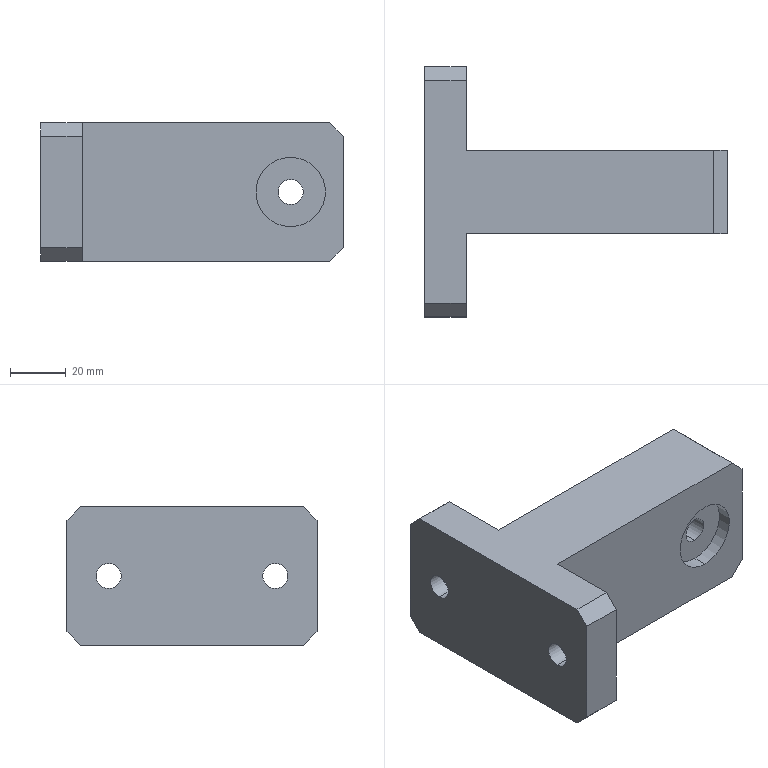Part | SolidWorks | features ICE 5, HoleWzd 3, Chamfer 1, Extrusion 1 | 1 solid | 31 faces | box 109 x 90 x 50 mm | volume 199011 mm3 | plane 19 | cylinder 12 | commonest cylinder face diameters 9 x6 15 x4 25 x2
STEP:
#1=CARTESIAN_POINT('',(6.,30.,7.5));
#2=VERTEX_POINT('',#1);
#3=CARTESIAN_POINT('',(6.,30.,-7.5));
#4=VERTEX_POINT('',#3);
#5=CARTESIAN_POINT('',(6.,30.,0.));
#6=DIRECTION('',(1.,0.,0.));
#7=DIRECTION('',(0.,0.,-1.));
#8=AXIS2_PLACEMENT_3D('',#5,#6,#7);
#9=CIRCLE('',#8,7.5);
#10=EDGE_CURVE('',#2,#4,#9,.T.);
#11=ORIENTED_EDGE('',*,*,#10,.F.);
#12=CARTESIAN_POINT('',(15.,30.,7.5));
#13=VERTEX_POINT('',#12);
#14=CARTESIAN_POINT('',(15.,30.,7.5));
#15=DIRECTION('',(1.,0.,0.));
#16=VECTOR('',#15,1000.);
#17=LINE('',#14,#16);
#18=EDGE_CURVE('',#2,#13,#17,.T.);
#19=ORIENTED_EDGE('',*,*,#18,.T.);
#20=CARTESIAN_POINT('',(15.,30.,-7.5));
#21=VERTEX_POINT('',#20);
#22=CARTESIAN_POINT('',(15.,30.,0.));
#23=DIRECTION('',(1.,0.,0.));
#24=DIRECTION('',(0.,0.,-1.));
#25=AXIS2_PLACEMENT_3D('',#22,#23,#24);
#26=CIRCLE('',#25,7.5);
#27=EDGE_CURVE('',#13,#21,#26,.T.);
#28=ORIENTED_EDGE('',*,*,#27,.T.);
#29=CARTESIAN_POINT('',(15.,30.,-7.5));
#30=DIRECTION('',(1.,0.,0.));
#31=VECTOR('',#30,1000.);
#32=LINE('',#29,#31);
#33=EDGE_CURVE('',#4,#21,#32,.T.);
#34=ORIENTED_EDGE('',*,*,#33,.F.);
#35=EDGE_LOOP('',(#11,#19,#28,#34));
#36=FACE_OUTER_BOUND('',#35,.T.);
#37=CARTESIAN_POINT('',(15.,30.,0.));
#38=DIRECTION('',(1.,0.,0.));
#39=DIRECTION('',(0.,0.,-1.));
#40=AXIS2_PLACEMENT_3D('',#37,#38,#39);
#41=CYLINDRICAL_SURFACE('',#40,7.5);
#42=ADVANCED_FACE('',(#36),#41,.F.);
#43=CARTESIAN_POINT('',(0.,30.,4.5));
#44=VERTEX_POINT('',#43);
#45=CARTESIAN_POINT('',(0.,30.,-4.5));
#46=VERTEX_POINT('',#45);
#47=CARTESIAN_POINT('',(0.,30.,0.));
#48=DIRECTION('',(1.,0.,0.));
#49=DIRECTION('',(0.,0.,-1.));
#50=AXIS2_PLACEMENT_3D('',#47,#48,#49);
#51=CIRCLE('',#50,4.5);
#52=EDGE_CURVE('',#44,#46,#51,.T.);
#53=ORIENTED_EDGE('',*,*,#52,.F.);
#54=CARTESIAN_POINT('',(6.,30.,4.5));
#55=VERTEX_POINT('',#54);
#56=CARTESIAN_POINT('',(15.,30.,4.5));
#57=DIRECTION('',(1.,0.,0.));
#58=VECTOR('',#57,1000.);
#59=LINE('',#56,#58);
#60=EDGE_CURVE('',#44,#55,#59,.T.);
#61=ORIENTED_EDGE('',*,*,#60,.T.);
#62=CARTESIAN_POINT('',(6.,30.,-4.5));
#63=VERTEX_POINT('',#62);
#64=CARTESIAN_POINT('',(6.,30.,0.));
#65=DIRECTION('',(1.,0.,0.));
#66=DIRECTION('',(0.,0.,-1.));
#67=AXIS2_PLACEMENT_3D('',#64,#65,#66);
#68=CIRCLE('',#67,4.5);
#69=EDGE_CURVE('',#55,#63,#68,.T.);
#70=ORIENTED_EDGE('',*,*,#69,.T.);
#71=CARTESIAN_POINT('',(15.,30.,-4.5));
#72=DIRECTION('',(1.,0.,0.));
#73=VECTOR('',#72,1000.);
#74=LINE('',#71,#73);
#75=EDGE_CURVE('',#46,#63,#74,.T.);
#76=ORIENTED_EDGE('',*,*,#75,.F.);
#77=EDGE_LOOP('',(#53,#61,#70,#76));
#78=FACE_OUTER_BOUND('',#77,.T.);
#79=CARTESIAN_POINT('',(15.,30.,0.));
#80=DIRECTION('',(1.,0.,0.));
#81=DIRECTION('',(0.,0.,-1.));
#82=AXIS2_PLACEMENT_3D('',#79,#80,#81);
#83=CYLINDRICAL_SURFACE('',#82,4.5);
#84=ADVANCED_FACE('',(#78),#83,.F.);
#85=CARTESIAN_POINT('',(6.,-30.,7.5));
#86=VERTEX_POINT('',#85);
#87=CARTESIAN_POINT('',(6.,-30.,-7.5));
#88=VERTEX_POINT('',#87);
#89=CARTESIAN_POINT('',(6.,-30.,0.));
#90=DIRECTION('',(1.,0.,0.));
#91=DIRECTION('',(0.,0.,-1.));
#92=AXIS2_PLACEMENT_3D('',#89,#90,#91);
#93=CIRCLE('',#92,7.5);
#94=EDGE_CURVE('',#86,#88,#93,.T.);
#95=ORIENTED_EDGE('',*,*,#94,.F.);
#96=CARTESIAN_POINT('',(15.,-30.,7.5));
#97=VERTEX_POINT('',#96);
#98=CARTESIAN_POINT('',(15.,-30.,7.5));
#99=DIRECTION('',(1.,0.,0.));
#100=VECTOR('',#99,1000.);
#101=LINE('',#98,#100);
#102=EDGE_CURVE('',#86,#97,#101,.T.);
#103=ORIENTED_EDGE('',*,*,#102,.T.);
#104=CARTESIAN_POINT('',(15.,-30.,-7.5));
#105=VERTEX_POINT('',#104);
#106=CARTESIAN_POINT('',(15.,-30.,0.));
#107=DIRECTION('',(1.,0.,0.));
#108=DIRECTION('',(0.,0.,-1.));
#109=AXIS2_PLACEMENT_3D('',#106,#107,#108);
#110=CIRCLE('',#109,7.5);
#111=EDGE_CURVE('',#97,#105,#110,.T.);
#112=ORIENTED_EDGE('',*,*,#111,.T.);
#113=CARTESIAN_POINT('',(15.,-30.,-7.5));
#114=DIRECTION('',(1.,0.,0.));
#115=VECTOR('',#114,1000.);
#116=LINE('',#113,#115);
#117=EDGE_CURVE('',#88,#105,#116,.T.);
#118=ORIENTED_EDGE('',*,*,#117,.F.);
#119=EDGE_LOOP('',(#95,#103,#112,#118));
#120=FACE_OUTER_BOUND('',#119,.T.);
#121=CARTESIAN_POINT('',(15.,-30.,0.));
#122=DIRECTION('',(1.,0.,0.));
#123=DIRECTION('',(0.,0.,-1.));
#124=AXIS2_PLACEMENT_3D('',#121,#122,#123);
#125=CYLINDRICAL_SURFACE('',#124,7.5);
#126=ADVANCED_FACE('',(#120),#125,.F.);
#127=CARTESIAN_POINT('',(0.,-30.,4.5));
#128=VERTEX_POINT('',#127);
#129=CARTESIAN_POINT('',(0.,-30.,-4.5));
#130=VERTEX_POINT('',#129);
#131=CARTESIAN_POINT('',(0.,-30.,0.));
#132=DIRECTION('',(1.,0.,0.));
#133=DIRECTION('',(0.,0.,-1.));
#134=AXIS2_PLACEMENT_3D('',#131,#132,#133);
#135=CIRCLE('',#134,4.5);
#136=EDGE_CURVE('',#128,#130,#135,.T.);
#137=ORIENTED_EDGE('',*,*,#136,.F.);
#138=CARTESIAN_POINT('',(6.,-30.,4.5));
#139=VERTEX_POINT('',#138);
#140=CARTESIAN_POINT('',(15.,-30.,4.5));
#141=DIRECTION('',(1.,0.,0.));
#142=VECTOR('',#141,1000.);
#143=LINE('',#140,#142);
#144=EDGE_CURVE('',#128,#139,#143,.T.);
#145=ORIENTED_EDGE('',*,*,#144,.T.);
#146=CARTESIAN_POINT('',(6.,-30.,-4.5));
#147=VERTEX_POINT('',#146);
#148=CARTESIAN_POINT('',(6.,-30.,0.));
#149=DIRECTION('',(1.,0.,0.));
#150=DIRECTION('',(0.,0.,-1.));
#151=AXIS2_PLACEMENT_3D('',#148,#149,#150);
#152=CIRCLE('',#151,4.5);
#153=EDGE_CURVE('',#139,#147,#152,.T.);
#154=ORIENTED_EDGE('',*,*,#153,.T.);
#155=CARTESIAN_POINT('',(15.,-30.,-4.5));
#156=DIRECTION('',(1.,0.,0.));
#157=VECTOR('',#156,1000.);
#158=LINE('',#155,#157);
#159=EDGE_CURVE('',#130,#147,#158,.T.);
#160=ORIENTED_EDGE('',*,*,#159,.F.);
#161=EDGE_LOOP('',(#137,#145,#154,#160));
#162=FACE_OUTER_BOUND('',#161,.T.);
#163=CARTESIAN_POINT('',(15.,-30.,0.));
#164=DIRECTION('',(1.,0.,0.));
#165=DIRECTION('',(0.,0.,-1.));
#166=AXIS2_PLACEMENT_3D('',#163,#164,#165);
#167=CYLINDRICAL_SURFACE('',#166,4.5);
#168=ADVANCED_FACE('',(#162),#167,.F.);
#169=CARTESIAN_POINT('',(90.,15.,4.5));
#170=VERTEX_POINT('',#169);
#171=CARTESIAN_POINT('',(90.,15.,-4.5));
#172=VERTEX_POINT('',#171);
#173=CARTESIAN_POINT('',(90.,15.,0.));
#174=DIRECTION('',(0.,-1.,0.));
#175=DIRECTION('',(0.,0.,-1.));
#176=AXIS2_PLACEMENT_3D('',#173,#174,#175);
#177=CIRCLE('',#176,4.5);
#178=EDGE_CURVE('',#170,#172,#177,.T.);
#179=ORIENTED_EDGE('',*,*,#178,.F.);
#180=CARTESIAN_POINT('',(90.,-10.,4.5));
#181=VERTEX_POINT('',#180);
#182=CARTESIAN_POINT('',(90.,-15.,4.5));
#183=DIRECTION('',(0.,-1.,0.));
#184=VECTOR('',#183,1000.);
#185=LINE('',#182,#184);
#186=EDGE_CURVE('',#170,#181,#185,.T.);
#187=ORIENTED_EDGE('',*,*,#186,.T.);
#188=CARTESIAN_POINT('',(90.,-10.,-4.5));
#189=VERTEX_POINT('',#188);
#190=CARTESIAN_POINT('',(90.,-10.,0.));
#191=DIRECTION('',(0.,-1.,0.));
#192=DIRECTION('',(0.,0.,-1.));
#193=AXIS2_PLACEMENT_3D('',#190,#191,#192);
#194=CIRCLE('',#193,4.5);
#195=EDGE_CURVE('',#181,#189,#194,.T.);
#196=ORIENTED_EDGE('',*,*,#195,.T.);
#197=CARTESIAN_POINT('',(90.,-15.,-4.5));
#198=DIRECTION('',(0.,-1.,0.));
#199=VECTOR('',#198,1000.);
#200=LINE('',#197,#199);
#201=EDGE_CURVE('',#172,#189,#200,.T.);
#202=ORIENTED_EDGE('',*,*,#201,.F.);
#203=EDGE_LOOP('',(#179,#187,#196,#202));
#204=FACE_OUTER_BOUND('',#203,.T.);
#205=CARTESIAN_POINT('',(90.,-15.,0.));
#206=DIRECTION('',(0.,-1.,0.));
#207=DIRECTION('',(0.,0.,-1.));
#208=AXIS2_PLACEMENT_3D('',#205,#206,#207);
#209=CYLINDRICAL_SURFACE('',#208,4.5);
#210=ADVANCED_FACE('',(#204),#209,.F.);
#211=CARTESIAN_POINT('',(90.,-10.,12.5));
#212=VERTEX_POINT('',#211);
#213=CARTESIAN_POINT('',(90.,-10.,-12.5));
#214=VERTEX_POINT('',#213);
#215=CARTESIAN_POINT('',(90.,-10.,0.));
#216=DIRECTION('',(0.,-1.,0.));
#217=DIRECTION('',(0.,0.,-1.));
#218=AXIS2_PLACEMENT_3D('',#215,#216,#217);
#219=CIRCLE('',#218,12.5);
#220=EDGE_CURVE('',#212,#214,#219,.T.);
#221=ORIENTED_EDGE('',*,*,#220,.F.);
#222=CARTESIAN_POINT('',(90.,-15.,12.5));
#223=VERTEX_POINT('',#222);
#224=CARTESIAN_POINT('',(90.,-10.,12.5));
#225=DIRECTION('',(0.,-1.,0.));
#226=VECTOR('',#225,1000.);
#227=LINE('',#224,#226);
#228=EDGE_CURVE('',#212,#223,#227,.T.);
#229=ORIENTED_EDGE('',*,*,#228,.T.);
#230=CARTESIAN_POINT('',(90.,-15.,-12.5));
#231=VERTEX_POINT('',#230);
#232=CARTESIAN_POINT('',(90.,-15.,0.));
#233=DIRECTION('',(0.,-1.,0.));
#234=DIRECTION('',(0.,0.,-1.));
#235=AXIS2_PLACEMENT_3D('',#232,#233,#234);
#236=CIRCLE('',#235,12.5);
#237=EDGE_CURVE('',#223,#231,#236,.T.);
#238=ORIENTED_EDGE('',*,*,#237,.T.);
#239=CARTESIAN_POINT('',(90.,-10.,-12.5));
#240=DIRECTION('',(0.,-1.,0.));
#241=VECTOR('',#240,1000.);
#242=LINE('',#239,#241);
#243=EDGE_CURVE('',#214,#231,#242,.T.);
#244=ORIENTED_EDGE('',*,*,#243,.F.);
#245=EDGE_LOOP('',(#221,#229,#238,#244));
#246=FACE_OUTER_BOUND('',#245,.T.);
#247=CARTESIAN_POINT('',(90.,-10.,0.));
#248=DIRECTION('',(0.,-1.,0.));
#249=DIRECTION('',(0.,0.,-1.));
#250=AXIS2_PLACEMENT_3D('',#247,#248,#249);
#251=CYLINDRICAL_SURFACE('',#250,12.5);
#252=ADVANCED_FACE('',(#246),#251,.F.);
#253=CARTESIAN_POINT('',(90.,15.,0.));
#254=DIRECTION('',(0.,-1.,0.));
#255=DIRECTION('',(0.,0.,-1.));
#256=AXIS2_PLACEMENT_3D('',#253,#254,#255);
#257=CIRCLE('',#256,4.5);
#258=EDGE_CURVE('',#172,#170,#257,.T.);
#259=ORIENTED_EDGE('',*,*,#258,.T.);
#260=ORIENTED_EDGE('',*,*,#178,.T.);
#261=EDGE_LOOP('',(#259,#260));
#262=FACE_BOUND('',#261,.T.);
#263=CARTESIAN_POINT('',(109.,15.,-20.));
#264=VERTEX_POINT('',#263);
#265=CARTESIAN_POINT('',(109.,15.,20.));
#266=VERTEX_POINT('',#265);
#267=CARTESIAN_POINT('',(109.,15.,25.));
#268=DIRECTION('',(0.,0.,1.));
#269=VECTOR('',#268,1000.);
#270=LINE('',#267,#269);
#271=EDGE_CURVE('',#264,#266,#270,.T.);
#272=ORIENTED_EDGE('',*,*,#271,.F.);
#273=CARTESIAN_POINT('',(104.,15.,-25.));
#274=VERTEX_POINT('',#273);
#275=CARTESIAN_POINT('',(109.,15.,-20.));
#276=DIRECTION('',(-0.7071,0.,-0.7071));
#277=VECTOR('',#276,1000.);
#278=LINE('',#275,#277);
#279=EDGE_CURVE('',#264,#274,#278,.T.);
#280=ORIENTED_EDGE('',*,*,#279,.T.);
#281=CARTESIAN_POINT('',(15.,15.,-25.));
#282=VERTEX_POINT('',#281);
#283=CARTESIAN_POINT('',(109.,15.,-25.));
#284=DIRECTION('',(-1.,0.,0.));
#285=VECTOR('',#284,1000.);
#286=LINE('',#283,#285);
#287=EDGE_CURVE('',#274,#282,#286,.T.);
#288=ORIENTED_EDGE('',*,*,#287,.T.);
#289=CARTESIAN_POINT('',(15.,15.,25.));
#290=VERTEX_POINT('',#289);
#291=CARTESIAN_POINT('',(15.,15.,-25.));
#292=DIRECTION('',(0.,0.,-1.));
#293=VECTOR('',#292,1000.);
#294=LINE('',#291,#293);
#295=EDGE_CURVE('',#290,#282,#294,.T.);
#296=ORIENTED_EDGE('',*,*,#295,.F.);
#297=CARTESIAN_POINT('',(104.,15.,25.));
#298=VERTEX_POINT('',#297);
#299=CARTESIAN_POINT('',(109.,15.,25.));
#300=DIRECTION('',(-1.,0.,0.));
#301=VECTOR('',#300,1000.);
#302=LINE('',#299,#301);
#303=EDGE_CURVE('',#298,#290,#302,.T.);
#304=ORIENTED_EDGE('',*,*,#303,.F.);
#305=CARTESIAN_POINT('',(109.,15.,20.));
#306=DIRECTION('',(0.7071,0.,-0.7071));
#307=VECTOR('',#306,1000.);
#308=LINE('',#305,#307);
#309=EDGE_CURVE('',#298,#266,#308,.T.);
#310=ORIENTED_EDGE('',*,*,#309,.T.);
#311=EDGE_LOOP('',(#272,#280,#288,#296,#304,#310));
#312=FACE_OUTER_BOUND('',#311,.T.);
#313=CARTESIAN_POINT('',(14.,15.,50.));
#314=DIRECTION('',(0.,-1.,0.));
#315=DIRECTION('',(0.,0.,-1.));
#316=AXIS2_PLACEMENT_3D('',#313,#314,#315);
#317=PLANE('',#316);
#318=ADVANCED_FACE('',(#262,#312),#317,.F.);
#319=CARTESIAN_POINT('',(90.,-15.,0.));
#320=DIRECTION('',(0.,-1.,0.));
#321=DIRECTION('',(0.,0.,-1.));
#322=AXIS2_PLACEMENT_3D('',#319,#320,#321);
#323=CIRCLE('',#322,12.5);
#324=EDGE_CURVE('',#231,#223,#323,.T.);
#325=ORIENTED_EDGE('',*,*,#324,.F.);
#326=ORIENTED_EDGE('',*,*,#237,.F.);
#327=EDGE_LOOP('',(#325,#326));
#328=FACE_BOUND('',#327,.T.);
#329=CARTESIAN_POINT('',(104.,-15.,-25.));
#330=VERTEX_POINT('',#329);
#331=CARTESIAN_POINT('',(15.,-15.,-25.));
#332=VERTEX_POINT('',#331);
#333=CARTESIAN_POINT('',(109.,-15.,-25.));
#334=DIRECTION('',(-1.,0.,0.));
#335=VECTOR('',#334,1000.);
#336=LINE('',#333,#335);
#337=EDGE_CURVE('',#330,#332,#336,.T.);
#338=ORIENTED_EDGE('',*,*,#337,.F.);
#339=CARTESIAN_POINT('',(109.,-15.,-20.));
#340=VERTEX_POINT('',#339);
#341=CARTESIAN_POINT('',(109.,-15.,-20.));
#342=DIRECTION('',(0.7071,0.,0.7071));
#343=VECTOR('',#342,1000.);
#344=LINE('',#341,#343);
#345=EDGE_CURVE('',#330,#340,#344,.T.);
#346=ORIENTED_EDGE('',*,*,#345,.T.);
#347=CARTESIAN_POINT('',(109.,-15.,20.));
#348=VERTEX_POINT('',#347);
#349=CARTESIAN_POINT('',(109.,-15.,25.));
#350=DIRECTION('',(0.,0.,-1.));
#351=VECTOR('',#350,1000.);
#352=LINE('',#349,#351);
#353=EDGE_CURVE('',#348,#340,#352,.T.);
#354=ORIENTED_EDGE('',*,*,#353,.F.);
#355=CARTESIAN_POINT('',(104.,-15.,25.));
#356=VERTEX_POINT('',#355);
#357=CARTESIAN_POINT('',(109.,-15.,20.));
#358=DIRECTION('',(-0.7071,0.,0.7071));
#359=VECTOR('',#358,1000.);
#360=LINE('',#357,#359);
#361=EDGE_CURVE('',#348,#356,#360,.T.);
#362=ORIENTED_EDGE('',*,*,#361,.T.);
#363=CARTESIAN_POINT('',(15.,-15.,25.));
#364=VERTEX_POINT('',#363);
#365=CARTESIAN_POINT('',(109.,-15.,25.));
#366=DIRECTION('',(-1.,0.,0.));
#367=VECTOR('',#366,1000.);
#368=LINE('',#365,#367);
#369=EDGE_CURVE('',#356,#364,#368,.T.);
#370=ORIENTED_EDGE('',*,*,#369,.T.);
#371=CARTESIAN_POINT('',(15.,-15.,25.));
#372=DIRECTION('',(0.,0.,1.));
#373=VECTOR('',#372,1000.);
#374=LINE('',#371,#373);
#375=EDGE_CURVE('',#332,#364,#374,.T.);
#376=ORIENTED_EDGE('',*,*,#375,.F.);
#377=EDGE_LOOP('',(#338,#346,#354,#362,#370,#376));
#378=FACE_OUTER_BOUND('',#377,.T.);
#379=CARTESIAN_POINT('',(14.,-15.,50.));
#380=DIRECTION('',(0.,1.,0.));
#381=DIRECTION('',(0.,0.,1.));
#382=AXIS2_PLACEMENT_3D('',#379,#380,#381);
#383=PLANE('',#382);
#384=ADVANCED_FACE('',(#328,#378),#383,.F.);
#385=CARTESIAN_POINT('',(0.,30.,0.));
#386=DIRECTION('',(1.,0.,0.));
#387=DIRECTION('',(0.,0.,-1.));
#388=AXIS2_PLACEMENT_3D('',#385,#386,#387);
#389=CIRCLE('',#388,4.5);
#390=EDGE_CURVE('',#46,#44,#389,.T.);
#391=ORIENTED_EDGE('',*,*,#390,.T.);
#392=ORIENTED_EDGE('',*,*,#52,.T.);
#393=EDGE_LOOP('',(#391,#392));
#394=FACE_BOUND('',#393,.T.);
#395=CARTESIAN_POINT('',(0.,-30.,0.));
#396=DIRECTION('',(1.,0.,0.));
#397=DIRECTION('',(0.,0.,-1.));
#398=AXIS2_PLACEMENT_3D('',#395,#396,#397);
#399=CIRCLE('',#398,4.5);
#400=EDGE_CURVE('',#130,#128,#399,.T.);
#401=ORIENTED_EDGE('',*,*,#400,.T.);
#402=ORIENTED_EDGE('',*,*,#136,.T.);
#403=EDGE_LOOP('',(#401,#402));
#404=FACE_BOUND('',#403,.T.);
#405=CARTESIAN_POINT('',(0.,40.,25.));
#406=VERTEX_POINT('',#405);
#407=CARTESIAN_POINT('',(0.,-40.,25.));
#408=VERTEX_POINT('',#407);
#409=CARTESIAN_POINT('',(0.,15.,25.));
#410=DIRECTION('',(0.,-1.,0.));
#411=VECTOR('',#410,1000.);
#412=LINE('',#409,#411);
#413=EDGE_CURVE('',#406,#408,#412,.T.);
#414=ORIENTED_EDGE('',*,*,#413,.F.);
#415=CARTESIAN_POINT('',(0.,45.,20.));
#416=VERTEX_POINT('',#415);
#417=CARTESIAN_POINT('',(0.,45.,20.));
#418=DIRECTION('',(0.,0.7071,-0.7071));
#419=VECTOR('',#418,1000.);
#420=LINE('',#417,#419);
#421=EDGE_CURVE('',#406,#416,#420,.T.);
#422=ORIENTED_EDGE('',*,*,#421,.T.);
#423=CARTESIAN_POINT('',(0.,45.,-20.));
#424=VERTEX_POINT('',#423);
#425=CARTESIAN_POINT('',(0.,45.,-25.));
#426=DIRECTION('',(0.,0.,1.));
#427=VECTOR('',#426,1000.);
#428=LINE('',#425,#427);
#429=EDGE_CURVE('',#424,#416,#428,.T.);
#430=ORIENTED_EDGE('',*,*,#429,.F.);
#431=CARTESIAN_POINT('',(0.,40.,-25.));
#432=VERTEX_POINT('',#431);
#433=CARTESIAN_POINT('',(0.,45.,-20.));
#434=DIRECTION('',(0.,-0.7071,-0.7071));
#435=VECTOR('',#434,1000.);
#436=LINE('',#433,#435);
#437=EDGE_CURVE('',#424,#432,#436,.T.);
#438=ORIENTED_EDGE('',*,*,#437,.T.);
#439=CARTESIAN_POINT('',(0.,-40.,-25.));
#440=VERTEX_POINT('',#439);
#441=CARTESIAN_POINT('',(0.,15.,-25.));
#442=DIRECTION('',(0.,1.,0.));
#443=VECTOR('',#442,1000.);
#444=LINE('',#441,#443);
#445=EDGE_CURVE('',#440,#432,#444,.T.);
#446=ORIENTED_EDGE('',*,*,#445,.F.);
#447=CARTESIAN_POINT('',(0.,-45.,-20.));
#448=VERTEX_POINT('',#447);
#449=CARTESIAN_POINT('',(0.,-45.,-20.));
#450=DIRECTION('',(0.,-0.7071,0.7071));
#451=VECTOR('',#450,1000.);
#452=LINE('',#449,#451);
#453=EDGE_CURVE('',#440,#448,#452,.T.);
#454=ORIENTED_EDGE('',*,*,#453,.T.);
#455=CARTESIAN_POINT('',(0.,-45.,20.));
#456=VERTEX_POINT('',#455);
#457=CARTESIAN_POINT('',(0.,-45.,25.));
#458=DIRECTION('',(0.,0.,-1.));
#459=VECTOR('',#458,1000.);
#460=LINE('',#457,#459);
#461=EDGE_CURVE('',#456,#448,#460,.T.);
#462=ORIENTED_EDGE('',*,*,#461,.F.);
#463=CARTESIAN_POINT('',(0.,-45.,20.));
#464=DIRECTION('',(0.,0.7071,0.7071));
#465=VECTOR('',#464,1000.);
#466=LINE('',#463,#465);
#467=EDGE_CURVE('',#456,#408,#466,.T.);
#468=ORIENTED_EDGE('',*,*,#467,.T.);
#469=EDGE_LOOP('',(#414,#422,#430,#438,#446,#454,#462,#468));
#470=FACE_OUTER_BOUND('',#469,.T.);
#471=CARTESIAN_POINT('',(0.,0.,0.));
#472=DIRECTION('',(1.,0.,0.));
#473=DIRECTION('',(0.,0.,-1.));
#474=AXIS2_PLACEMENT_3D('',#471,#472,#473);
#475=PLANE('',#474);
#476=ADVANCED_FACE('',(#394,#404,#470),#475,.F.);
#477=ORIENTED_EDGE('',*,*,#445,.T.);
#478=CARTESIAN_POINT('',(15.,40.,-25.));
#479=VERTEX_POINT('',#478);
#480=CARTESIAN_POINT('',(15.,40.,-25.));
#481=DIRECTION('',(1.,0.,0.));
#482=VECTOR('',#481,1000.);
#483=LINE('',#480,#482);
#484=EDGE_CURVE('',#432,#479,#483,.T.);
#485=ORIENTED_EDGE('',*,*,#484,.T.);
#486=CARTESIAN_POINT('',(15.,45.,-25.));
#487=DIRECTION('',(0.,-1.,0.));
#488=VECTOR('',#487,1000.);
#489=LINE('',#486,#488);
#490=EDGE_CURVE('',#479,#282,#489,.T.);
#491=ORIENTED_EDGE('',*,*,#490,.T.);
#492=ORIENTED_EDGE('',*,*,#287,.F.);
#493=CARTESIAN_POINT('',(104.,-15.,-25.));
#494=DIRECTION('',(0.,-1.,0.));
#495=VECTOR('',#494,1000.);
#496=LINE('',#493,#495);
#497=EDGE_CURVE('',#274,#330,#496,.T.);
#498=ORIENTED_EDGE('',*,*,#497,.T.);
#499=ORIENTED_EDGE('',*,*,#337,.T.);
#500=CARTESIAN_POINT('',(15.,-40.,-25.));
#501=VERTEX_POINT('',#500);
#502=CARTESIAN_POINT('',(15.,-45.,-25.));
#503=DIRECTION('',(0.,1.,0.));
#504=VECTOR('',#503,1000.);
#505=LINE('',#502,#504);
#506=EDGE_CURVE('',#501,#332,#505,.T.);
#507=ORIENTED_EDGE('',*,*,#506,.F.);
#508=CARTESIAN_POINT('',(0.,-40.,-25.));
#509=DIRECTION('',(-1.,0.,0.));
#510=VECTOR('',#509,1000.);
#511=LINE('',#508,#510);
#512=EDGE_CURVE('',#501,#440,#511,.T.);
#513=ORIENTED_EDGE('',*,*,#512,.T.);
#514=EDGE_LOOP('',(#477,#485,#491,#492,#498,#499,#507,#513));
#515=FACE_OUTER_BOUND('',#514,.T.);
#516=CARTESIAN_POINT('',(109.,15.,-25.));
#517=DIRECTION('',(0.,0.,1.));
#518=DIRECTION('',(1.,0.,0.));
#519=AXIS2_PLACEMENT_3D('',#516,#517,#518);
#520=PLANE('',#519);
#521=ADVANCED_FACE('',(#515),#520,.F.);
#522=CARTESIAN_POINT('',(15.,40.,25.));
#523=VERTEX_POINT('',#522);
#524=CARTESIAN_POINT('',(15.,45.,25.));
#525=DIRECTION('',(0.,-1.,0.));
#526=VECTOR('',#525,1000.);
#527=LINE('',#524,#526);
#528=EDGE_CURVE('',#523,#290,#527,.T.);
#529=ORIENTED_EDGE('',*,*,#528,.F.);
#530=CARTESIAN_POINT('',(0.,40.,25.));
#531=DIRECTION('',(-1.,0.,0.));
#532=VECTOR('',#531,1000.);
#533=LINE('',#530,#532);
#534=EDGE_CURVE('',#523,#406,#533,.T.);
#535=ORIENTED_EDGE('',*,*,#534,.T.);
#536=ORIENTED_EDGE('',*,*,#413,.T.);
#537=CARTESIAN_POINT('',(15.,-40.,25.));
#538=VERTEX_POINT('',#537);
#539=CARTESIAN_POINT('',(15.,-40.,25.));
#540=DIRECTION('',(1.,0.,0.));
#541=VECTOR('',#540,1000.);
#542=LINE('',#539,#541);
#543=EDGE_CURVE('',#408,#538,#542,.T.);
#544=ORIENTED_EDGE('',*,*,#543,.T.);
#545=CARTESIAN_POINT('',(15.,-45.,25.));
#546=DIRECTION('',(0.,1.,0.));
#547=VECTOR('',#546,1000.);
#548=LINE('',#545,#547);
#549=EDGE_CURVE('',#538,#364,#548,.T.);
#550=ORIENTED_EDGE('',*,*,#549,.T.);
#551=ORIENTED_EDGE('',*,*,#369,.F.);
#552=CARTESIAN_POINT('',(104.,15.,25.));
#553=DIRECTION('',(0.,1.,0.));
#554=VECTOR('',#553,1000.);
#555=LINE('',#552,#554);
#556=EDGE_CURVE('',#356,#298,#555,.T.);
#557=ORIENTED_EDGE('',*,*,#556,.T.);
#558=ORIENTED_EDGE('',*,*,#303,.T.);
#559=EDGE_LOOP('',(#529,#535,#536,#544,#550,#551,#557,#558));
#560=FACE_OUTER_BOUND('',#559,.T.);
#561=CARTESIAN_POINT('',(109.,15.,25.));
#562=DIRECTION('',(0.,0.,-1.));
#563=DIRECTION('',(-1.,0.,0.));
#564=AXIS2_PLACEMENT_3D('',#561,#562,#563);
#565=PLANE('',#564);
#566=ADVANCED_FACE('',(#560),#565,.F.);
#567=ORIENTED_EDGE('',*,*,#353,.T.);
#568=CARTESIAN_POINT('',(109.,15.,-20.));
#569=DIRECTION('',(0.,1.,0.));
#570=VECTOR('',#569,1000.);
#571=LINE('',#568,#570);
#572=EDGE_CURVE('',#340,#264,#571,.T.);
#573=ORIENTED_EDGE('',*,*,#572,.T.);
#574=ORIENTED_EDGE('',*,*,#271,.T.);
#575=CARTESIAN_POINT('',(109.,-15.,20.));
#576=DIRECTION('',(0.,-1.,0.));
#577=VECTOR('',#576,1000.);
#578=LINE('',#575,#577);
#579=EDGE_CURVE('',#266,#348,#578,.T.);
#580=ORIENTED_EDGE('',*,*,#579,.T.);
#581=EDGE_LOOP('',(#567,#573,#574,#580));
#582=FACE_OUTER_BOUND('',#581,.T.);
#583=CARTESIAN_POINT('',(109.,0.,0.));
#584=DIRECTION('',(1.,0.,0.));
#585=DIRECTION('',(0.,0.,-1.));
#586=AXIS2_PLACEMENT_3D('',#583,#584,#585);
#587=PLANE('',#586);
#588=ADVANCED_FACE('',(#582),#587,.T.);
#589=ORIENTED_EDGE('',*,*,#228,.F.);
#590=CARTESIAN_POINT('',(90.,-10.,0.));
#591=DIRECTION('',(0.,-1.,0.));
#592=DIRECTION('',(0.,0.,-1.));
#593=AXIS2_PLACEMENT_3D('',#590,#591,#592);
#594=CIRCLE('',#593,12.5);
#595=EDGE_CURVE('',#214,#212,#594,.T.);
#596=ORIENTED_EDGE('',*,*,#595,.F.);
#597=ORIENTED_EDGE('',*,*,#243,.T.);
#598=ORIENTED_EDGE('',*,*,#324,.T.);
#599=EDGE_LOOP('',(#589,#596,#597,#598));
#600=FACE_OUTER_BOUND('',#599,.T.);
#601=CARTESIAN_POINT('',(90.,-10.,0.));
#602=DIRECTION('',(0.,-1.,0.));
#603=DIRECTION('',(0.,0.,-1.));
#604=AXIS2_PLACEMENT_3D('',#601,#602,#603);
#605=CYLINDRICAL_SURFACE('',#604,12.5);
#606=ADVANCED_FACE('',(#600),#605,.F.);
#607=CARTESIAN_POINT('',(90.,-10.,0.));
#608=DIRECTION('',(0.,-1.,0.));
#609=DIRECTION('',(0.,0.,-1.));
#610=AXIS2_PLACEMENT_3D('',#607,#608,#609);
#611=CIRCLE('',#610,4.5);
#612=EDGE_CURVE('',#189,#181,#611,.T.);
#613=ORIENTED_EDGE('',*,*,#612,.F.);
#614=ORIENTED_EDGE('',*,*,#195,.F.);
#615=EDGE_LOOP('',(#613,#614));
#616=FACE_BOUND('',#615,.T.);
#617=ORIENTED_EDGE('',*,*,#595,.T.);
#618=ORIENTED_EDGE('',*,*,#220,.T.);
#619=EDGE_LOOP('',(#617,#618));
#620=FACE_OUTER_BOUND('',#619,.T.);
#621=CARTESIAN_POINT('',(90.,-10.,0.));
#622=DIRECTION('',(0.,-1.,0.));
#623=DIRECTION('',(0.,0.,-1.));
#624=AXIS2_PLACEMENT_3D('',#621,#622,#623);
#625=PLANE('',#624);
#626=ADVANCED_FACE('',(#616,#620),#625,.T.);
#627=ORIENTED_EDGE('',*,*,#186,.F.);
#628=ORIENTED_EDGE('',*,*,#258,.F.);
#629=ORIENTED_EDGE('',*,*,#201,.T.);
#630=ORIENTED_EDGE('',*,*,#612,.T.);
#631=EDGE_LOOP('',(#627,#628,#629,#630));
#632=FACE_OUTER_BOUND('',#631,.T.);
#633=CARTESIAN_POINT('',(90.,-15.,0.));
#634=DIRECTION('',(0.,-1.,0.));
#635=DIRECTION('',(0.,0.,-1.));
#636=AXIS2_PLACEMENT_3D('',#633,#634,#635);
#637=CYLINDRICAL_SURFACE('',#636,4.5);
#638=ADVANCED_FACE('',(#632),#637,.F.);
#639=CARTESIAN_POINT('',(15.,-30.,0.));
#640=DIRECTION('',(1.,0.,0.));
#641=DIRECTION('',(0.,0.,-1.));
#642=AXIS2_PLACEMENT_3D('',#639,#640,#641);
#643=CIRCLE('',#642,7.5);
#644=EDGE_CURVE('',#105,#97,#643,.T.);
#645=ORIENTED_EDGE('',*,*,#644,.F.);
#646=ORIENTED_EDGE('',*,*,#111,.F.);
#647=EDGE_LOOP('',(#645,#646));
#648=FACE_BOUND('',#647,.T.);
#649=ORIENTED_EDGE('',*,*,#549,.F.);
#650=CARTESIAN_POINT('',(15.,-45.,20.));
#651=VERTEX_POINT('',#650);
#652=CARTESIAN_POINT('',(15.,-45.,20.));
#653=DIRECTION('',(0.,-0.7071,-0.7071));
#654=VECTOR('',#653,1000.);
#655=LINE('',#652,#654);
#656=EDGE_CURVE('',#538,#651,#655,.T.);
#657=ORIENTED_EDGE('',*,*,#656,.T.);
#658=CARTESIAN_POINT('',(15.,-45.,-20.));
#659=VERTEX_POINT('',#658);
#660=CARTESIAN_POINT('',(15.,-45.,25.));
#661=DIRECTION('',(0.,0.,1.));
#662=VECTOR('',#661,1000.);
#663=LINE('',#660,#662);
#664=EDGE_CURVE('',#659,#651,#663,.T.);
#665=ORIENTED_EDGE('',*,*,#664,.F.);
#666=CARTESIAN_POINT('',(15.,-45.,-20.));
#667=DIRECTION('',(0.,0.7071,-0.7071));
#668=VECTOR('',#667,1000.);
#669=LINE('',#666,#668);
#670=EDGE_CURVE('',#659,#501,#669,.T.);
#671=ORIENTED_EDGE('',*,*,#670,.T.);
#672=ORIENTED_EDGE('',*,*,#506,.T.);
#673=ORIENTED_EDGE('',*,*,#375,.T.);
#674=EDGE_LOOP('',(#649,#657,#665,#671,#672,#673));
#675=FACE_OUTER_BOUND('',#674,.T.);
#676=CARTESIAN_POINT('',(15.,-45.,25.));
#677=DIRECTION('',(-1.,0.,0.));
#678=DIRECTION('',(0.,0.,1.));
#679=AXIS2_PLACEMENT_3D('',#676,#677,#678);
#680=PLANE('',#679);
#681=ADVANCED_FACE('',(#648,#675),#680,.F.);
#682=ORIENTED_EDGE('',*,*,#664,.T.);
#683=CARTESIAN_POINT('',(0.,-45.,20.));
#684=DIRECTION('',(-1.,0.,0.));
#685=VECTOR('',#684,1000.);
#686=LINE('',#683,#685);
#687=EDGE_CURVE('',#651,#456,#686,.T.);
#688=ORIENTED_EDGE('',*,*,#687,.T.);
#689=ORIENTED_EDGE('',*,*,#461,.T.);
#690=CARTESIAN_POINT('',(15.,-45.,-20.));
#691=DIRECTION('',(1.,0.,0.));
#692=VECTOR('',#691,1000.);
#693=LINE('',#690,#692);
#694=EDGE_CURVE('',#448,#659,#693,.T.);
#695=ORIENTED_EDGE('',*,*,#694,.T.);
#696=EDGE_LOOP('',(#682,#688,#689,#695));
#697=FACE_OUTER_BOUND('',#696,.T.);
#698=CARTESIAN_POINT('',(0.,-45.,0.));
#699=DIRECTION('',(0.,-1.,0.));
#700=DIRECTION('',(0.,0.,-1.));
#701=AXIS2_PLACEMENT_3D('',#698,#699,#700);
#702=PLANE('',#701);
#703=ADVANCED_FACE('',(#697),#702,.T.);
#704=CARTESIAN_POINT('',(15.,30.,0.));
#705=DIRECTION('',(1.,0.,0.));
#706=DIRECTION('',(0.,0.,-1.));
#707=AXIS2_PLACEMENT_3D('',#704,#705,#706);
#708=CIRCLE('',#707,7.5);
#709=EDGE_CURVE('',#21,#13,#708,.T.);
#710=ORIENTED_EDGE('',*,*,#709,.F.);
#711=ORIENTED_EDGE('',*,*,#27,.F.);
#712=EDGE_LOOP('',(#710,#711));
#713=FACE_BOUND('',#712,.T.);
#714=CARTESIAN_POINT('',(15.,45.,20.));
#715=VERTEX_POINT('',#714);
#716=CARTESIAN_POINT('',(15.,45.,-20.));
#717=VERTEX_POINT('',#716);
#718=CARTESIAN_POINT('',(15.,45.,-25.));
#719=DIRECTION('',(0.,0.,-1.));
#720=VECTOR('',#719,1000.);
#721=LINE('',#718,#720);
#722=EDGE_CURVE('',#715,#717,#721,.T.);
#723=ORIENTED_EDGE('',*,*,#722,.F.);
#724=CARTESIAN_POINT('',(15.,45.,20.));
#725=DIRECTION('',(0.,-0.7071,0.7071));
#726=VECTOR('',#725,1000.);
#727=LINE('',#724,#726);
#728=EDGE_CURVE('',#715,#523,#727,.T.);
#729=ORIENTED_EDGE('',*,*,#728,.T.);
#730=ORIENTED_EDGE('',*,*,#528,.T.);
#731=ORIENTED_EDGE('',*,*,#295,.T.);
#732=ORIENTED_EDGE('',*,*,#490,.F.);
#733=CARTESIAN_POINT('',(15.,45.,-20.));
#734=DIRECTION('',(0.,0.7071,0.7071));
#735=VECTOR('',#734,1000.);
#736=LINE('',#733,#735);
#737=EDGE_CURVE('',#479,#717,#736,.T.);
#738=ORIENTED_EDGE('',*,*,#737,.T.);
#739=EDGE_LOOP('',(#723,#729,#730,#731,#732,#738));
#740=FACE_OUTER_BOUND('',#739,.T.);
#741=CARTESIAN_POINT('',(15.,45.,-25.));
#742=DIRECTION('',(-1.,0.,0.));
#743=DIRECTION('',(0.,0.,1.));
#744=AXIS2_PLACEMENT_3D('',#741,#742,#743);
#745=PLANE('',#744);
#746=ADVANCED_FACE('',(#713,#740),#745,.F.);
#747=ORIENTED_EDGE('',*,*,#429,.T.);
#748=CARTESIAN_POINT('',(15.,45.,20.));
#749=DIRECTION('',(1.,0.,0.));
#750=VECTOR('',#749,1000.);
#751=LINE('',#748,#750);
#752=EDGE_CURVE('',#416,#715,#751,.T.);
#753=ORIENTED_EDGE('',*,*,#752,.T.);
#754=ORIENTED_EDGE('',*,*,#722,.T.);
#755=CARTESIAN_POINT('',(0.,45.,-20.));
#756=DIRECTION('',(-1.,0.,0.));
#757=VECTOR('',#756,1000.);
#758=LINE('',#755,#757);
#759=EDGE_CURVE('',#717,#424,#758,.T.);
#760=ORIENTED_EDGE('',*,*,#759,.T.);
#761=EDGE_LOOP('',(#747,#753,#754,#760));
#762=FACE_OUTER_BOUND('',#761,.T.);
#763=CARTESIAN_POINT('',(0.,45.,0.));
#764=DIRECTION('',(0.,1.,0.));
#765=DIRECTION('',(0.,0.,1.));
#766=AXIS2_PLACEMENT_3D('',#763,#764,#765);
#767=PLANE('',#766);
#768=ADVANCED_FACE('',(#762),#767,.T.);
#769=ORIENTED_EDGE('',*,*,#144,.F.);
#770=ORIENTED_EDGE('',*,*,#400,.F.);
#771=ORIENTED_EDGE('',*,*,#159,.T.);
#772=CARTESIAN_POINT('',(6.,-30.,0.));
#773=DIRECTION('',(1.,0.,0.));
#774=DIRECTION('',(0.,0.,-1.));
#775=AXIS2_PLACEMENT_3D('',#772,#773,#774);
#776=CIRCLE('',#775,4.5);
#777=EDGE_CURVE('',#147,#139,#776,.T.);
#778=ORIENTED_EDGE('',*,*,#777,.T.);
#779=EDGE_LOOP('',(#769,#770,#771,#778));
#780=FACE_OUTER_BOUND('',#779,.T.);
#781=CARTESIAN_POINT('',(15.,-30.,0.));
#782=DIRECTION('',(1.,0.,0.));
#783=DIRECTION('',(0.,0.,-1.));
#784=AXIS2_PLACEMENT_3D('',#781,#782,#783);
#785=CYLINDRICAL_SURFACE('',#784,4.5);
#786=ADVANCED_FACE('',(#780),#785,.F.);
#787=ORIENTED_EDGE('',*,*,#777,.F.);
#788=ORIENTED_EDGE('',*,*,#153,.F.);
#789=EDGE_LOOP('',(#787,#788));
#790=FACE_BOUND('',#789,.T.);
#791=CARTESIAN_POINT('',(6.,-30.,0.));
#792=DIRECTION('',(1.,0.,0.));
#793=DIRECTION('',(0.,0.,-1.));
#794=AXIS2_PLACEMENT_3D('',#791,#792,#793);
#795=CIRCLE('',#794,7.5);
#796=EDGE_CURVE('',#88,#86,#795,.T.);
#797=ORIENTED_EDGE('',*,*,#796,.T.);
#798=ORIENTED_EDGE('',*,*,#94,.T.);
#799=EDGE_LOOP('',(#797,#798));
#800=FACE_OUTER_BOUND('',#799,.T.);
#801=CARTESIAN_POINT('',(6.,-25.5,0.));
#802=DIRECTION('',(-1.,0.,0.));
#803=DIRECTION('',(0.,0.,1.));
#804=AXIS2_PLACEMENT_3D('',#801,#802,#803);
#805=PLANE('',#804);
#806=ADVANCED_FACE('',(#790,#800),#805,.F.);
#807=ORIENTED_EDGE('',*,*,#102,.F.);
#808=ORIENTED_EDGE('',*,*,#796,.F.);
#809=ORIENTED_EDGE('',*,*,#117,.T.);
#810=ORIENTED_EDGE('',*,*,#644,.T.);
#811=EDGE_LOOP('',(#807,#808,#809,#810));
#812=FACE_OUTER_BOUND('',#811,.T.);
#813=CARTESIAN_POINT('',(15.,-30.,0.));
#814=DIRECTION('',(1.,0.,0.));
#815=DIRECTION('',(0.,0.,-1.));
#816=AXIS2_PLACEMENT_3D('',#813,#814,#815);
#817=CYLINDRICAL_SURFACE('',#816,7.5);
#818=ADVANCED_FACE('',(#812),#817,.F.);
#819=ORIENTED_EDGE('',*,*,#60,.F.);
#820=ORIENTED_EDGE('',*,*,#390,.F.);
#821=ORIENTED_EDGE('',*,*,#75,.T.);
#822=CARTESIAN_POINT('',(6.,30.,0.));
#823=DIRECTION('',(1.,0.,0.));
#824=DIRECTION('',(0.,0.,-1.));
#825=AXIS2_PLACEMENT_3D('',#822,#823,#824);
#826=CIRCLE('',#825,4.5);
#827=EDGE_CURVE('',#63,#55,#826,.T.);
#828=ORIENTED_EDGE('',*,*,#827,.T.);
#829=EDGE_LOOP('',(#819,#820,#821,#828));
#830=FACE_OUTER_BOUND('',#829,.T.);
#831=CARTESIAN_POINT('',(15.,30.,0.));
#832=DIRECTION('',(1.,0.,0.));
#833=DIRECTION('',(0.,0.,-1.));
#834=AXIS2_PLACEMENT_3D('',#831,#832,#833);
#835=CYLINDRICAL_SURFACE('',#834,4.5);
#836=ADVANCED_FACE('',(#830),#835,.F.);
#837=ORIENTED_EDGE('',*,*,#827,.F.);
#838=ORIENTED_EDGE('',*,*,#69,.F.);
#839=EDGE_LOOP('',(#837,#838));
#840=FACE_BOUND('',#839,.T.);
#841=CARTESIAN_POINT('',(6.,30.,0.));
#842=DIRECTION('',(1.,0.,0.));
#843=DIRECTION('',(0.,0.,-1.));
#844=AXIS2_PLACEMENT_3D('',#841,#842,#843);
#845=CIRCLE('',#844,7.5);
#846=EDGE_CURVE('',#4,#2,#845,.T.);
#847=ORIENTED_EDGE('',*,*,#846,.T.);
#848=ORIENTED_EDGE('',*,*,#10,.T.);
#849=EDGE_LOOP('',(#847,#848));
#850=FACE_OUTER_BOUND('',#849,.T.);
#851=CARTESIAN_POINT('',(6.,34.5,0.));
#852=DIRECTION('',(-1.,0.,0.));
#853=DIRECTION('',(0.,0.,1.));
#854=AXIS2_PLACEMENT_3D('',#851,#852,#853);
#855=PLANE('',#854);
#856=ADVANCED_FACE('',(#840,#850),#855,.F.);
#857=ORIENTED_EDGE('',*,*,#18,.F.);
#858=ORIENTED_EDGE('',*,*,#846,.F.);
#859=ORIENTED_EDGE('',*,*,#33,.T.);
#860=ORIENTED_EDGE('',*,*,#709,.T.);
#861=EDGE_LOOP('',(#857,#858,#859,#860));
#862=FACE_OUTER_BOUND('',#861,.T.);
#863=CARTESIAN_POINT('',(15.,30.,0.));
#864=DIRECTION('',(1.,0.,0.));
#865=DIRECTION('',(0.,0.,-1.));
#866=AXIS2_PLACEMENT_3D('',#863,#864,#865);
#867=CYLINDRICAL_SURFACE('',#866,7.5);
#868=ADVANCED_FACE('',(#862),#867,.F.);
#869=ORIENTED_EDGE('',*,*,#421,.F.);
#870=ORIENTED_EDGE('',*,*,#534,.F.);
#871=ORIENTED_EDGE('',*,*,#728,.F.);
#872=ORIENTED_EDGE('',*,*,#752,.F.);
#873=EDGE_LOOP('',(#869,#870,#871,#872));
#874=FACE_OUTER_BOUND('',#873,.T.);
#875=CARTESIAN_POINT('',(0.,45.,20.));
#876=DIRECTION('',(0.,0.7071,0.7071));
#877=DIRECTION('',(-1.,0.,0.));
#878=AXIS2_PLACEMENT_3D('',#875,#876,#877);
#879=PLANE('',#878);
#880=ADVANCED_FACE('',(#874),#879,.T.);
#881=ORIENTED_EDGE('',*,*,#737,.F.);
#882=ORIENTED_EDGE('',*,*,#484,.F.);
#883=ORIENTED_EDGE('',*,*,#437,.F.);
#884=ORIENTED_EDGE('',*,*,#759,.F.);
#885=EDGE_LOOP('',(#881,#882,#883,#884));
#886=FACE_OUTER_BOUND('',#885,.T.);
#887=CARTESIAN_POINT('',(0.,45.,-20.));
#888=DIRECTION('',(0.,0.7071,-0.7071));
#889=DIRECTION('',(1.,0.,0.));
#890=AXIS2_PLACEMENT_3D('',#887,#888,#889);
#891=PLANE('',#890);
#892=ADVANCED_FACE('',(#886),#891,.T.);
#893=ORIENTED_EDGE('',*,*,#656,.F.);
#894=ORIENTED_EDGE('',*,*,#543,.F.);
#895=ORIENTED_EDGE('',*,*,#467,.F.);
#896=ORIENTED_EDGE('',*,*,#687,.F.);
#897=EDGE_LOOP('',(#893,#894,#895,#896));
#898=FACE_OUTER_BOUND('',#897,.T.);
#899=CARTESIAN_POINT('',(0.,-45.,20.));
#900=DIRECTION('',(0.,-0.7071,0.7071));
#901=DIRECTION('',(1.,0.,0.));
#902=AXIS2_PLACEMENT_3D('',#899,#900,#901);
#903=PLANE('',#902);
#904=ADVANCED_FACE('',(#898),#903,.T.);
#905=ORIENTED_EDGE('',*,*,#453,.F.);
#906=ORIENTED_EDGE('',*,*,#512,.F.);
#907=ORIENTED_EDGE('',*,*,#670,.F.);
#908=ORIENTED_EDGE('',*,*,#694,.F.);
#909=EDGE_LOOP('',(#905,#906,#907,#908));
#910=FACE_OUTER_BOUND('',#909,.T.);
#911=CARTESIAN_POINT('',(0.,-45.,-20.));
#912=DIRECTION('',(0.,-0.7071,-0.7071));
#913=DIRECTION('',(-1.,0.,0.));
#914=AXIS2_PLACEMENT_3D('',#911,#912,#913);
#915=PLANE('',#914);
#916=ADVANCED_FACE('',(#910),#915,.T.);
#917=ORIENTED_EDGE('',*,*,#345,.F.);
#918=ORIENTED_EDGE('',*,*,#497,.F.);
#919=ORIENTED_EDGE('',*,*,#279,.F.);
#920=ORIENTED_EDGE('',*,*,#572,.F.);
#921=EDGE_LOOP('',(#917,#918,#919,#920));
#922=FACE_OUTER_BOUND('',#921,.T.);
#923=CARTESIAN_POINT('',(109.,0.,-20.));
#924=DIRECTION('',(0.7071,0.,-0.7071));
#925=DIRECTION('',(0.,-1.,0.));
#926=AXIS2_PLACEMENT_3D('',#923,#924,#925);
#927=PLANE('',#926);
#928=ADVANCED_FACE('',(#922),#927,.T.);
#929=ORIENTED_EDGE('',*,*,#309,.F.);
#930=ORIENTED_EDGE('',*,*,#556,.F.);
#931=ORIENTED_EDGE('',*,*,#361,.F.);
#932=ORIENTED_EDGE('',*,*,#579,.F.);
#933=EDGE_LOOP('',(#929,#930,#931,#932));
#934=FACE_OUTER_BOUND('',#933,.T.);
#935=CARTESIAN_POINT('',(109.,0.,20.));
#936=DIRECTION('',(0.7071,0.,0.7071));
#937=DIRECTION('',(0.,1.,0.));
#938=AXIS2_PLACEMENT_3D('',#935,#936,#937);
#939=PLANE('',#938);
#940=ADVANCED_FACE('',(#934),#939,.T.);
#941=CLOSED_SHELL('',(#42,#84,#126,#168,#210,#252,#318,#384,#476,#521,#566,#588,#606,#626,#638,#681,#703,#746,#768,#786,#806,#818,#836,#856,#868,#880,#892,#904,#916,#928,#940));
#942=MANIFOLD_SOLID_BREP('',#941);
#943=CARTESIAN_POINT('',(0.,0.,0.));
#944=DIRECTION('',(0.,0.,1.));
#945=DIRECTION('',(1.,0.,0.));
#946=AXIS2_PLACEMENT_3D('',#943,#944,#945);
#947=(LENGTH_UNIT()NAMED_UNIT(*)SI_UNIT(.MILLI.,.METRE.));
#948=UNCERTAINTY_MEASURE_WITH_UNIT(LENGTH_MEASURE(0.00001),#947,'','');
#949=(NAMED_UNIT(*)PLANE_ANGLE_UNIT()SI_UNIT($,.RADIAN.));
#950=(NAMED_UNIT(*)SI_UNIT($,.STERADIAN.)SOLID_ANGLE_UNIT());
#951=(GEOMETRIC_REPRESENTATION_CONTEXT(3)GLOBAL_UNCERTAINTY_ASSIGNED_CONTEXT((#948))GLOBAL_UNIT_ASSIGNED_CONTEXT((#947,#949,#950))REPRESENTATION_CONTEXT('',''));
#952=ADVANCED_BREP_SHAPE_REPRESENTATION('',(#942,#946),#951);